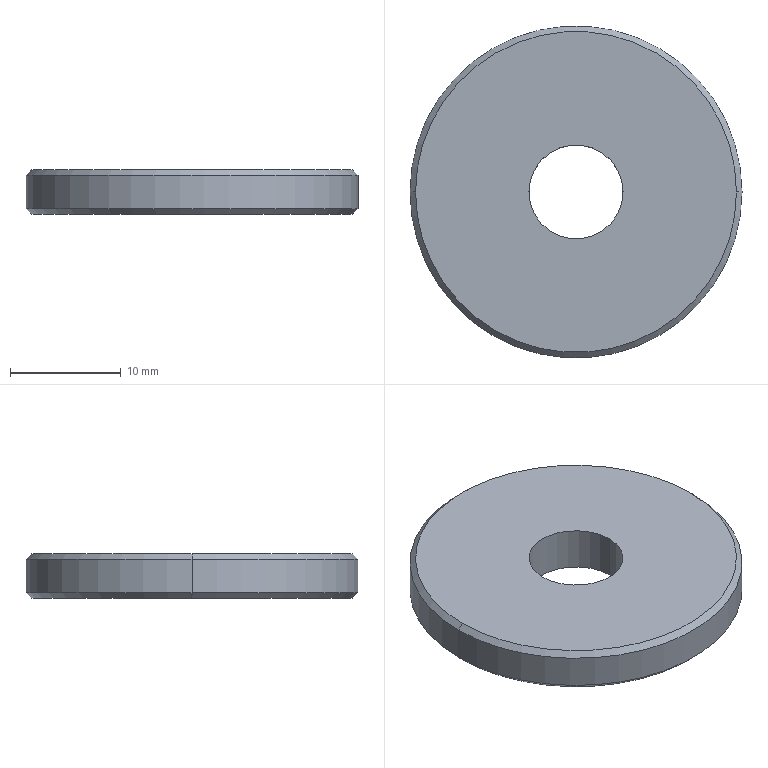Part | STEP file | 11-FG-Z01211 | 1 solid | 10 faces | box 30 x 30 x 4 mm | volume 2577 mm3 | cone 4 | cylinder 4 | plane 2 | commonest cylinder face diameters 8.5 x2 30 x2
STEP:
#1=CARTESIAN_POINT('',(14.5,0.,4.));
#2=VERTEX_POINT('',#1);
#3=CARTESIAN_POINT('',(-14.5,0.,4.));
#4=VERTEX_POINT('',#3);
#5=CARTESIAN_POINT('',(0.,0.,4.));
#6=DIRECTION('',(0.,0.,1.));
#7=DIRECTION('',(1.,0.,0.));
#8=AXIS2_PLACEMENT_3D('',#5,#6,#7);
#9=CIRCLE('',#8,14.5);
#10=EDGE_CURVE('',#2,#4,#9,.T.);
#11=ORIENTED_EDGE('',*,*,#10,.F.);
#12=CARTESIAN_POINT('',(15.,0.,3.5));
#13=VERTEX_POINT('',#12);
#14=CARTESIAN_POINT('',(14.5,0.,4.));
#15=DIRECTION('',(0.7071,0.,-0.7071));
#16=VECTOR('',#15,1000.);
#17=LINE('',#14,#16);
#18=EDGE_CURVE('',#2,#13,#17,.T.);
#19=ORIENTED_EDGE('',*,*,#18,.T.);
#20=CARTESIAN_POINT('',(-15.,0.,3.5));
#21=VERTEX_POINT('',#20);
#22=CARTESIAN_POINT('',(0.,0.,3.5));
#23=DIRECTION('',(0.,0.,-1.));
#24=DIRECTION('',(1.,0.,0.));
#25=AXIS2_PLACEMENT_3D('',#22,#23,#24);
#26=CIRCLE('',#25,15.);
#27=EDGE_CURVE('',#21,#13,#26,.T.);
#28=ORIENTED_EDGE('',*,*,#27,.F.);
#29=CARTESIAN_POINT('',(-14.5,0.,4.));
#30=DIRECTION('',(-0.7071,0.,-0.7071));
#31=VECTOR('',#30,1000.);
#32=LINE('',#29,#31);
#33=EDGE_CURVE('',#4,#21,#32,.T.);
#34=ORIENTED_EDGE('',*,*,#33,.F.);
#35=EDGE_LOOP('',(#11,#19,#28,#34));
#36=FACE_OUTER_BOUND('',#35,.T.);
#37=CARTESIAN_POINT('',(0.,0.,4.));
#38=DIRECTION('',(0.,0.,-1.));
#39=DIRECTION('',(-1.,0.,0.));
#40=AXIS2_PLACEMENT_3D('',#37,#38,#39);
#41=CONICAL_SURFACE('',#40,14.5,0.7854);
#42=ADVANCED_FACE('',(#36),#41,.T.);
#43=CARTESIAN_POINT('',(-14.5,0.,0.));
#44=VERTEX_POINT('',#43);
#45=CARTESIAN_POINT('',(14.5,0.,0.));
#46=VERTEX_POINT('',#45);
#47=CARTESIAN_POINT('',(0.,0.,0.));
#48=DIRECTION('',(0.,0.,-1.));
#49=DIRECTION('',(1.,0.,0.));
#50=AXIS2_PLACEMENT_3D('',#47,#48,#49);
#51=CIRCLE('',#50,14.5);
#52=EDGE_CURVE('',#44,#46,#51,.T.);
#53=ORIENTED_EDGE('',*,*,#52,.F.);
#54=CARTESIAN_POINT('',(-15.,0.,0.5));
#55=VERTEX_POINT('',#54);
#56=CARTESIAN_POINT('',(-15.,0.,0.5));
#57=DIRECTION('',(-0.7071,0.,0.7071));
#58=VECTOR('',#57,1000.);
#59=LINE('',#56,#58);
#60=EDGE_CURVE('',#44,#55,#59,.T.);
#61=ORIENTED_EDGE('',*,*,#60,.T.);
#62=CARTESIAN_POINT('',(15.,0.,0.5));
#63=VERTEX_POINT('',#62);
#64=CARTESIAN_POINT('',(0.,0.,0.5));
#65=DIRECTION('',(0.,0.,1.));
#66=DIRECTION('',(1.,0.,0.));
#67=AXIS2_PLACEMENT_3D('',#64,#65,#66);
#68=CIRCLE('',#67,15.);
#69=EDGE_CURVE('',#63,#55,#68,.T.);
#70=ORIENTED_EDGE('',*,*,#69,.F.);
#71=CARTESIAN_POINT('',(15.,0.,0.5));
#72=DIRECTION('',(0.7071,0.,0.7071));
#73=VECTOR('',#72,1000.);
#74=LINE('',#71,#73);
#75=EDGE_CURVE('',#46,#63,#74,.T.);
#76=ORIENTED_EDGE('',*,*,#75,.F.);
#77=EDGE_LOOP('',(#53,#61,#70,#76));
#78=FACE_OUTER_BOUND('',#77,.T.);
#79=CARTESIAN_POINT('',(0.,0.,0.5));
#80=DIRECTION('',(0.,0.,1.));
#81=DIRECTION('',(1.,0.,0.));
#82=AXIS2_PLACEMENT_3D('',#79,#80,#81);
#83=CONICAL_SURFACE('',#82,15.,0.7854);
#84=ADVANCED_FACE('',(#78),#83,.T.);
#85=CARTESIAN_POINT('',(-4.25,0.,4.));
#86=VERTEX_POINT('',#85);
#87=CARTESIAN_POINT('',(4.25,0.,4.));
#88=VERTEX_POINT('',#87);
#89=CARTESIAN_POINT('',(0.,0.,4.));
#90=DIRECTION('',(0.,0.,1.));
#91=DIRECTION('',(1.,0.,0.));
#92=AXIS2_PLACEMENT_3D('',#89,#90,#91);
#93=CIRCLE('',#92,4.25);
#94=EDGE_CURVE('',#86,#88,#93,.T.);
#95=ORIENTED_EDGE('',*,*,#94,.T.);
#96=CARTESIAN_POINT('',(4.25,0.,0.));
#97=VERTEX_POINT('',#96);
#98=CARTESIAN_POINT('',(4.25,0.,4.));
#99=DIRECTION('',(0.,0.,-1.));
#100=VECTOR('',#99,1000.);
#101=LINE('',#98,#100);
#102=EDGE_CURVE('',#88,#97,#101,.T.);
#103=ORIENTED_EDGE('',*,*,#102,.T.);
#104=CARTESIAN_POINT('',(-4.25,0.,0.));
#105=VERTEX_POINT('',#104);
#106=CARTESIAN_POINT('',(0.,0.,0.));
#107=DIRECTION('',(0.,0.,1.));
#108=DIRECTION('',(1.,0.,0.));
#109=AXIS2_PLACEMENT_3D('',#106,#107,#108);
#110=CIRCLE('',#109,4.25);
#111=EDGE_CURVE('',#105,#97,#110,.T.);
#112=ORIENTED_EDGE('',*,*,#111,.F.);
#113=CARTESIAN_POINT('',(-4.25,0.,4.));
#114=DIRECTION('',(0.,0.,-1.));
#115=VECTOR('',#114,1000.);
#116=LINE('',#113,#115);
#117=EDGE_CURVE('',#86,#105,#116,.T.);
#118=ORIENTED_EDGE('',*,*,#117,.F.);
#119=EDGE_LOOP('',(#95,#103,#112,#118));
#120=FACE_OUTER_BOUND('',#119,.T.);
#121=CARTESIAN_POINT('',(0.,0.,4.));
#122=DIRECTION('',(0.,0.,-1.));
#123=DIRECTION('',(-1.,0.,0.));
#124=AXIS2_PLACEMENT_3D('',#121,#122,#123);
#125=CYLINDRICAL_SURFACE('',#124,4.25);
#126=ADVANCED_FACE('',(#120),#125,.F.);
#127=ORIENTED_EDGE('',*,*,#27,.T.);
#128=CARTESIAN_POINT('',(15.,0.,4.));
#129=DIRECTION('',(0.,0.,-1.));
#130=VECTOR('',#129,1000.);
#131=LINE('',#128,#130);
#132=EDGE_CURVE('',#13,#63,#131,.T.);
#133=ORIENTED_EDGE('',*,*,#132,.T.);
#134=ORIENTED_EDGE('',*,*,#69,.T.);
#135=CARTESIAN_POINT('',(-15.,0.,4.));
#136=DIRECTION('',(0.,0.,-1.));
#137=VECTOR('',#136,1000.);
#138=LINE('',#135,#137);
#139=EDGE_CURVE('',#21,#55,#138,.T.);
#140=ORIENTED_EDGE('',*,*,#139,.F.);
#141=EDGE_LOOP('',(#127,#133,#134,#140));
#142=FACE_OUTER_BOUND('',#141,.T.);
#143=CARTESIAN_POINT('',(0.,0.,4.));
#144=DIRECTION('',(0.,0.,-1.));
#145=DIRECTION('',(-1.,0.,0.));
#146=AXIS2_PLACEMENT_3D('',#143,#144,#145);
#147=CYLINDRICAL_SURFACE('',#146,15.);
#148=ADVANCED_FACE('',(#142),#147,.T.);
#149=CARTESIAN_POINT('',(0.,0.,4.));
#150=DIRECTION('',(0.,0.,1.));
#151=DIRECTION('',(1.,0.,0.));
#152=AXIS2_PLACEMENT_3D('',#149,#150,#151);
#153=CIRCLE('',#152,14.5);
#154=EDGE_CURVE('',#4,#2,#153,.T.);
#155=ORIENTED_EDGE('',*,*,#154,.T.);
#156=ORIENTED_EDGE('',*,*,#10,.T.);
#157=EDGE_LOOP('',(#155,#156));
#158=FACE_OUTER_BOUND('',#157,.T.);
#159=ORIENTED_EDGE('',*,*,#94,.F.);
#160=CARTESIAN_POINT('',(0.,0.,4.));
#161=DIRECTION('',(0.,0.,1.));
#162=DIRECTION('',(1.,0.,0.));
#163=AXIS2_PLACEMENT_3D('',#160,#161,#162);
#164=CIRCLE('',#163,4.25);
#165=EDGE_CURVE('',#88,#86,#164,.T.);
#166=ORIENTED_EDGE('',*,*,#165,.F.);
#167=EDGE_LOOP('',(#159,#166));
#168=FACE_BOUND('',#167,.T.);
#169=CARTESIAN_POINT('',(0.,0.,4.));
#170=DIRECTION('',(0.,0.,1.));
#171=DIRECTION('',(1.,0.,0.));
#172=AXIS2_PLACEMENT_3D('',#169,#170,#171);
#173=PLANE('',#172);
#174=ADVANCED_FACE('',(#158,#168),#173,.T.);
#175=CARTESIAN_POINT('',(0.,0.,0.));
#176=DIRECTION('',(0.,0.,-1.));
#177=DIRECTION('',(1.,0.,0.));
#178=AXIS2_PLACEMENT_3D('',#175,#176,#177);
#179=CIRCLE('',#178,14.5);
#180=EDGE_CURVE('',#46,#44,#179,.T.);
#181=ORIENTED_EDGE('',*,*,#180,.T.);
#182=ORIENTED_EDGE('',*,*,#52,.T.);
#183=EDGE_LOOP('',(#181,#182));
#184=FACE_OUTER_BOUND('',#183,.T.);
#185=ORIENTED_EDGE('',*,*,#111,.T.);
#186=CARTESIAN_POINT('',(0.,0.,0.));
#187=DIRECTION('',(0.,0.,1.));
#188=DIRECTION('',(1.,0.,0.));
#189=AXIS2_PLACEMENT_3D('',#186,#187,#188);
#190=CIRCLE('',#189,4.25);
#191=EDGE_CURVE('',#97,#105,#190,.T.);
#192=ORIENTED_EDGE('',*,*,#191,.T.);
#193=EDGE_LOOP('',(#185,#192));
#194=FACE_BOUND('',#193,.T.);
#195=CARTESIAN_POINT('',(0.,0.,0.));
#196=DIRECTION('',(0.,0.,1.));
#197=DIRECTION('',(1.,0.,0.));
#198=AXIS2_PLACEMENT_3D('',#195,#196,#197);
#199=PLANE('',#198);
#200=ADVANCED_FACE('',(#184,#194),#199,.F.);
#201=ORIENTED_EDGE('',*,*,#132,.F.);
#202=CARTESIAN_POINT('',(0.,0.,3.5));
#203=DIRECTION('',(0.,0.,-1.));
#204=DIRECTION('',(1.,0.,0.));
#205=AXIS2_PLACEMENT_3D('',#202,#203,#204);
#206=CIRCLE('',#205,15.);
#207=EDGE_CURVE('',#13,#21,#206,.T.);
#208=ORIENTED_EDGE('',*,*,#207,.T.);
#209=ORIENTED_EDGE('',*,*,#139,.T.);
#210=CARTESIAN_POINT('',(0.,0.,0.5));
#211=DIRECTION('',(0.,0.,1.));
#212=DIRECTION('',(1.,0.,0.));
#213=AXIS2_PLACEMENT_3D('',#210,#211,#212);
#214=CIRCLE('',#213,15.);
#215=EDGE_CURVE('',#55,#63,#214,.T.);
#216=ORIENTED_EDGE('',*,*,#215,.T.);
#217=EDGE_LOOP('',(#201,#208,#209,#216));
#218=FACE_OUTER_BOUND('',#217,.T.);
#219=CARTESIAN_POINT('',(0.,0.,4.));
#220=DIRECTION('',(0.,0.,-1.));
#221=DIRECTION('',(-1.,0.,0.));
#222=AXIS2_PLACEMENT_3D('',#219,#220,#221);
#223=CYLINDRICAL_SURFACE('',#222,15.);
#224=ADVANCED_FACE('',(#218),#223,.T.);
#225=ORIENTED_EDGE('',*,*,#102,.F.);
#226=ORIENTED_EDGE('',*,*,#165,.T.);
#227=ORIENTED_EDGE('',*,*,#117,.T.);
#228=ORIENTED_EDGE('',*,*,#191,.F.);
#229=EDGE_LOOP('',(#225,#226,#227,#228));
#230=FACE_OUTER_BOUND('',#229,.T.);
#231=CARTESIAN_POINT('',(0.,0.,4.));
#232=DIRECTION('',(0.,0.,-1.));
#233=DIRECTION('',(-1.,0.,0.));
#234=AXIS2_PLACEMENT_3D('',#231,#232,#233);
#235=CYLINDRICAL_SURFACE('',#234,4.25);
#236=ADVANCED_FACE('',(#230),#235,.F.);
#237=ORIENTED_EDGE('',*,*,#60,.F.);
#238=ORIENTED_EDGE('',*,*,#180,.F.);
#239=ORIENTED_EDGE('',*,*,#75,.T.);
#240=ORIENTED_EDGE('',*,*,#215,.F.);
#241=EDGE_LOOP('',(#237,#238,#239,#240));
#242=FACE_OUTER_BOUND('',#241,.T.);
#243=CARTESIAN_POINT('',(0.,0.,0.5));
#244=DIRECTION('',(0.,0.,1.));
#245=DIRECTION('',(1.,0.,0.));
#246=AXIS2_PLACEMENT_3D('',#243,#244,#245);
#247=CONICAL_SURFACE('',#246,15.,0.7854);
#248=ADVANCED_FACE('',(#242),#247,.T.);
#249=ORIENTED_EDGE('',*,*,#18,.F.);
#250=ORIENTED_EDGE('',*,*,#154,.F.);
#251=ORIENTED_EDGE('',*,*,#33,.T.);
#252=ORIENTED_EDGE('',*,*,#207,.F.);
#253=EDGE_LOOP('',(#249,#250,#251,#252));
#254=FACE_OUTER_BOUND('',#253,.T.);
#255=CARTESIAN_POINT('',(0.,0.,4.));
#256=DIRECTION('',(0.,0.,-1.));
#257=DIRECTION('',(-1.,0.,0.));
#258=AXIS2_PLACEMENT_3D('',#255,#256,#257);
#259=CONICAL_SURFACE('',#258,14.5,0.7854);
#260=ADVANCED_FACE('',(#254),#259,.T.);
#261=CLOSED_SHELL('',(#42,#84,#126,#148,#174,#200,#224,#236,#248,#260));
#262=MANIFOLD_SOLID_BREP('',#261);
#263=CARTESIAN_POINT('',(0.,0.,0.));
#264=DIRECTION('',(0.,0.,1.));
#265=DIRECTION('',(1.,0.,0.));
#266=AXIS2_PLACEMENT_3D('',#263,#264,#265);
#267=(LENGTH_UNIT()NAMED_UNIT(*)SI_UNIT(.MILLI.,.METRE.));
#268=UNCERTAINTY_MEASURE_WITH_UNIT(LENGTH_MEASURE(0.00001),#267,'','');
#269=(NAMED_UNIT(*)PLANE_ANGLE_UNIT()SI_UNIT($,.RADIAN.));
#270=(NAMED_UNIT(*)SI_UNIT($,.STERADIAN.)SOLID_ANGLE_UNIT());
#271=(GEOMETRIC_REPRESENTATION_CONTEXT(3)GLOBAL_UNCERTAINTY_ASSIGNED_CONTEXT((#268))GLOBAL_UNIT_ASSIGNED_CONTEXT((#267,#269,#270))REPRESENTATION_CONTEXT('',''));
#272=ADVANCED_BREP_SHAPE_REPRESENTATION('',(#262,#266),#271);